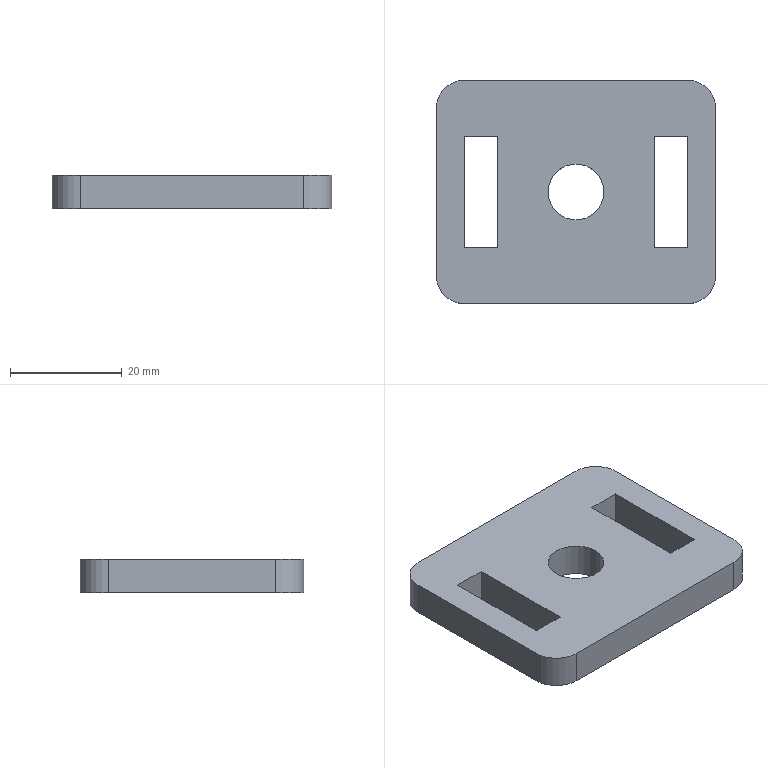Part | SolidWorks | features FlatPattern 1, SMBaseFlange 1, SheetMetal 1 | 1 solid | 20 faces | box 50 x 40 x 6 mm | volume 9960 mm3 | plane 14 | cylinder 6 | commonest cylinder face diameters 10 x6
STEP:
#1=CARTESIAN_POINT('',(-172.,0.,6.));
#2=VERTEX_POINT('',#1);
#3=CARTESIAN_POINT('',(-162.,0.,6.));
#4=VERTEX_POINT('',#3);
#5=CARTESIAN_POINT('',(-167.,0.,6.));
#6=DIRECTION('',(0.,0.,1.));
#7=DIRECTION('',(1.,0.,0.));
#8=AXIS2_PLACEMENT_3D('',#5,#6,#7);
#9=CIRCLE('',#8,5.);
#10=EDGE_CURVE('',#2,#4,#9,.T.);
#11=ORIENTED_EDGE('',*,*,#10,.T.);
#12=CARTESIAN_POINT('',(-162.,0.,0.));
#13=VERTEX_POINT('',#12);
#14=CARTESIAN_POINT('',(-162.,0.,6.));
#15=DIRECTION('',(0.,0.,-1.));
#16=VECTOR('',#15,1000.);
#17=LINE('',#14,#16);
#18=EDGE_CURVE('',#4,#13,#17,.T.);
#19=ORIENTED_EDGE('',*,*,#18,.T.);
#20=CARTESIAN_POINT('',(-172.,0.,0.));
#21=VERTEX_POINT('',#20);
#22=CARTESIAN_POINT('',(-167.,0.,0.));
#23=DIRECTION('',(0.,0.,1.));
#24=DIRECTION('',(1.,0.,0.));
#25=AXIS2_PLACEMENT_3D('',#22,#23,#24);
#26=CIRCLE('',#25,5.);
#27=EDGE_CURVE('',#21,#13,#26,.T.);
#28=ORIENTED_EDGE('',*,*,#27,.F.);
#29=CARTESIAN_POINT('',(-172.,0.,6.));
#30=DIRECTION('',(0.,0.,-1.));
#31=VECTOR('',#30,1000.);
#32=LINE('',#29,#31);
#33=EDGE_CURVE('',#2,#21,#32,.T.);
#34=ORIENTED_EDGE('',*,*,#33,.F.);
#35=EDGE_LOOP('',(#11,#19,#28,#34));
#36=FACE_OUTER_BOUND('',#35,.T.);
#37=CARTESIAN_POINT('',(-167.,0.,6.));
#38=DIRECTION('',(0.,0.,-1.));
#39=DIRECTION('',(-1.,0.,0.));
#40=AXIS2_PLACEMENT_3D('',#37,#38,#39);
#41=CYLINDRICAL_SURFACE('',#40,5.);
#42=ADVANCED_FACE('',(#36),#41,.F.);
#43=CARTESIAN_POINT('',(-147.,-20.,6.));
#44=VERTEX_POINT('',#43);
#45=CARTESIAN_POINT('',(-142.,-15.,6.));
#46=VERTEX_POINT('',#45);
#47=CARTESIAN_POINT('',(-147.,-15.,6.));
#48=DIRECTION('',(0.,0.,1.));
#49=DIRECTION('',(1.,0.,0.));
#50=AXIS2_PLACEMENT_3D('',#47,#48,#49);
#51=CIRCLE('',#50,5.);
#52=EDGE_CURVE('',#44,#46,#51,.T.);
#53=ORIENTED_EDGE('',*,*,#52,.T.);
#54=CARTESIAN_POINT('',(-142.,15.,6.));
#55=VERTEX_POINT('',#54);
#56=CARTESIAN_POINT('',(-142.,15.,6.));
#57=DIRECTION('',(0.,1.,0.));
#58=VECTOR('',#57,1000.);
#59=LINE('',#56,#58);
#60=EDGE_CURVE('',#46,#55,#59,.T.);
#61=ORIENTED_EDGE('',*,*,#60,.T.);
#62=CARTESIAN_POINT('',(-147.,20.,6.));
#63=VERTEX_POINT('',#62);
#64=CARTESIAN_POINT('',(-147.,15.,6.));
#65=DIRECTION('',(0.,0.,1.));
#66=DIRECTION('',(-1.,0.,0.));
#67=AXIS2_PLACEMENT_3D('',#64,#65,#66);
#68=CIRCLE('',#67,5.);
#69=EDGE_CURVE('',#55,#63,#68,.T.);
#70=ORIENTED_EDGE('',*,*,#69,.T.);
#71=CARTESIAN_POINT('',(-187.,20.,6.));
#72=VERTEX_POINT('',#71);
#73=CARTESIAN_POINT('',(-187.,20.,6.));
#74=DIRECTION('',(-1.,0.,0.));
#75=VECTOR('',#74,1000.);
#76=LINE('',#73,#75);
#77=EDGE_CURVE('',#63,#72,#76,.T.);
#78=ORIENTED_EDGE('',*,*,#77,.T.);
#79=CARTESIAN_POINT('',(-192.,15.,6.));
#80=VERTEX_POINT('',#79);
#81=CARTESIAN_POINT('',(-187.,15.,6.));
#82=DIRECTION('',(0.,0.,1.));
#83=DIRECTION('',(1.,0.,0.));
#84=AXIS2_PLACEMENT_3D('',#81,#82,#83);
#85=CIRCLE('',#84,5.);
#86=EDGE_CURVE('',#72,#80,#85,.T.);
#87=ORIENTED_EDGE('',*,*,#86,.T.);
#88=CARTESIAN_POINT('',(-192.,-15.,6.));
#89=VERTEX_POINT('',#88);
#90=CARTESIAN_POINT('',(-192.,15.,6.));
#91=DIRECTION('',(0.,-1.,0.));
#92=VECTOR('',#91,1000.);
#93=LINE('',#90,#92);
#94=EDGE_CURVE('',#80,#89,#93,.T.);
#95=ORIENTED_EDGE('',*,*,#94,.T.);
#96=CARTESIAN_POINT('',(-187.,-20.,6.));
#97=VERTEX_POINT('',#96);
#98=CARTESIAN_POINT('',(-187.,-15.,6.));
#99=DIRECTION('',(0.,0.,1.));
#100=DIRECTION('',(1.,0.,0.));
#101=AXIS2_PLACEMENT_3D('',#98,#99,#100);
#102=CIRCLE('',#101,5.);
#103=EDGE_CURVE('',#89,#97,#102,.T.);
#104=ORIENTED_EDGE('',*,*,#103,.T.);
#105=CARTESIAN_POINT('',(-187.,-20.,6.));
#106=DIRECTION('',(1.,0.,0.));
#107=VECTOR('',#106,1000.);
#108=LINE('',#105,#107);
#109=EDGE_CURVE('',#97,#44,#108,.T.);
#110=ORIENTED_EDGE('',*,*,#109,.T.);
#111=EDGE_LOOP('',(#53,#61,#70,#78,#87,#95,#104,#110));
#112=FACE_OUTER_BOUND('',#111,.T.);
#113=ORIENTED_EDGE('',*,*,#10,.F.);
#114=CARTESIAN_POINT('',(-167.,0.,6.));
#115=DIRECTION('',(0.,0.,1.));
#116=DIRECTION('',(1.,0.,0.));
#117=AXIS2_PLACEMENT_3D('',#114,#115,#116);
#118=CIRCLE('',#117,5.);
#119=EDGE_CURVE('',#4,#2,#118,.T.);
#120=ORIENTED_EDGE('',*,*,#119,.F.);
#121=EDGE_LOOP('',(#113,#120));
#122=FACE_BOUND('',#121,.T.);
#123=CARTESIAN_POINT('',(-181.,10.,6.));
#124=VERTEX_POINT('',#123);
#125=CARTESIAN_POINT('',(-187.,10.,6.));
#126=VERTEX_POINT('',#125);
#127=CARTESIAN_POINT('',(-181.,10.,6.));
#128=DIRECTION('',(-1.,0.,0.));
#129=VECTOR('',#128,1000.);
#130=LINE('',#127,#129);
#131=EDGE_CURVE('',#124,#126,#130,.T.);
#132=ORIENTED_EDGE('',*,*,#131,.F.);
#133=CARTESIAN_POINT('',(-181.,-10.,6.));
#134=VERTEX_POINT('',#133);
#135=CARTESIAN_POINT('',(-181.,10.,6.));
#136=DIRECTION('',(0.,1.,0.));
#137=VECTOR('',#136,1000.);
#138=LINE('',#135,#137);
#139=EDGE_CURVE('',#134,#124,#138,.T.);
#140=ORIENTED_EDGE('',*,*,#139,.F.);
#141=CARTESIAN_POINT('',(-187.,-10.,6.));
#142=VERTEX_POINT('',#141);
#143=CARTESIAN_POINT('',(-181.,-10.,6.));
#144=DIRECTION('',(1.,0.,0.));
#145=VECTOR('',#144,1000.);
#146=LINE('',#143,#145);
#147=EDGE_CURVE('',#142,#134,#146,.T.);
#148=ORIENTED_EDGE('',*,*,#147,.F.);
#149=CARTESIAN_POINT('',(-187.,10.,6.));
#150=DIRECTION('',(0.,-1.,0.));
#151=VECTOR('',#150,1000.);
#152=LINE('',#149,#151);
#153=EDGE_CURVE('',#126,#142,#152,.T.);
#154=ORIENTED_EDGE('',*,*,#153,.F.);
#155=EDGE_LOOP('',(#132,#140,#148,#154));
#156=FACE_BOUND('',#155,.T.);
#157=CARTESIAN_POINT('',(-153.,-10.,6.));
#158=VERTEX_POINT('',#157);
#159=CARTESIAN_POINT('',(-147.,-10.,6.));
#160=VERTEX_POINT('',#159);
#161=CARTESIAN_POINT('',(-153.,-10.,6.));
#162=DIRECTION('',(1.,0.,0.));
#163=VECTOR('',#162,1000.);
#164=LINE('',#161,#163);
#165=EDGE_CURVE('',#158,#160,#164,.T.);
#166=ORIENTED_EDGE('',*,*,#165,.F.);
#167=CARTESIAN_POINT('',(-153.,10.,6.));
#168=VERTEX_POINT('',#167);
#169=CARTESIAN_POINT('',(-153.,10.,6.));
#170=DIRECTION('',(0.,-1.,0.));
#171=VECTOR('',#170,1000.);
#172=LINE('',#169,#171);
#173=EDGE_CURVE('',#168,#158,#172,.T.);
#174=ORIENTED_EDGE('',*,*,#173,.F.);
#175=CARTESIAN_POINT('',(-147.,10.,6.));
#176=VERTEX_POINT('',#175);
#177=CARTESIAN_POINT('',(-153.,10.,6.));
#178=DIRECTION('',(-1.,0.,0.));
#179=VECTOR('',#178,1000.);
#180=LINE('',#177,#179);
#181=EDGE_CURVE('',#176,#168,#180,.T.);
#182=ORIENTED_EDGE('',*,*,#181,.F.);
#183=CARTESIAN_POINT('',(-147.,10.,6.));
#184=DIRECTION('',(0.,1.,0.));
#185=VECTOR('',#184,1000.);
#186=LINE('',#183,#185);
#187=EDGE_CURVE('',#160,#176,#186,.T.);
#188=ORIENTED_EDGE('',*,*,#187,.F.);
#189=EDGE_LOOP('',(#166,#174,#182,#188));
#190=FACE_BOUND('',#189,.T.);
#191=CARTESIAN_POINT('',(-147.,-15.,6.));
#192=DIRECTION('',(0.,0.,1.));
#193=DIRECTION('',(1.,0.,0.));
#194=AXIS2_PLACEMENT_3D('',#191,#192,#193);
#195=PLANE('',#194);
#196=ADVANCED_FACE('',(#112,#122,#156,#190),#195,.T.);
#197=CARTESIAN_POINT('',(-181.,-10.,0.));
#198=VERTEX_POINT('',#197);
#199=CARTESIAN_POINT('',(-181.,10.,0.));
#200=VERTEX_POINT('',#199);
#201=CARTESIAN_POINT('',(-181.,10.,0.));
#202=DIRECTION('',(0.,1.,0.));
#203=VECTOR('',#202,1000.);
#204=LINE('',#201,#203);
#205=EDGE_CURVE('',#198,#200,#204,.T.);
#206=ORIENTED_EDGE('',*,*,#205,.T.);
#207=CARTESIAN_POINT('',(-187.,10.,0.));
#208=VERTEX_POINT('',#207);
#209=CARTESIAN_POINT('',(-181.,10.,0.));
#210=DIRECTION('',(-1.,0.,0.));
#211=VECTOR('',#210,1000.);
#212=LINE('',#209,#211);
#213=EDGE_CURVE('',#200,#208,#212,.T.);
#214=ORIENTED_EDGE('',*,*,#213,.T.);
#215=CARTESIAN_POINT('',(-187.,-10.,0.));
#216=VERTEX_POINT('',#215);
#217=CARTESIAN_POINT('',(-187.,10.,0.));
#218=DIRECTION('',(0.,-1.,0.));
#219=VECTOR('',#218,1000.);
#220=LINE('',#217,#219);
#221=EDGE_CURVE('',#208,#216,#220,.T.);
#222=ORIENTED_EDGE('',*,*,#221,.T.);
#223=CARTESIAN_POINT('',(-181.,-10.,0.));
#224=DIRECTION('',(1.,0.,0.));
#225=VECTOR('',#224,1000.);
#226=LINE('',#223,#225);
#227=EDGE_CURVE('',#216,#198,#226,.T.);
#228=ORIENTED_EDGE('',*,*,#227,.T.);
#229=EDGE_LOOP('',(#206,#214,#222,#228));
#230=FACE_BOUND('',#229,.T.);
#231=CARTESIAN_POINT('',(-147.,-20.,0.));
#232=VERTEX_POINT('',#231);
#233=CARTESIAN_POINT('',(-142.,-15.,0.));
#234=VERTEX_POINT('',#233);
#235=CARTESIAN_POINT('',(-147.,-15.,0.));
#236=DIRECTION('',(0.,0.,1.));
#237=DIRECTION('',(1.,0.,0.));
#238=AXIS2_PLACEMENT_3D('',#235,#236,#237);
#239=CIRCLE('',#238,5.);
#240=EDGE_CURVE('',#232,#234,#239,.T.);
#241=ORIENTED_EDGE('',*,*,#240,.F.);
#242=CARTESIAN_POINT('',(-187.,-20.,0.));
#243=VERTEX_POINT('',#242);
#244=CARTESIAN_POINT('',(-187.,-20.,0.));
#245=DIRECTION('',(1.,0.,0.));
#246=VECTOR('',#245,1000.);
#247=LINE('',#244,#246);
#248=EDGE_CURVE('',#243,#232,#247,.T.);
#249=ORIENTED_EDGE('',*,*,#248,.F.);
#250=CARTESIAN_POINT('',(-192.,-15.,0.));
#251=VERTEX_POINT('',#250);
#252=CARTESIAN_POINT('',(-187.,-15.,0.));
#253=DIRECTION('',(0.,0.,1.));
#254=DIRECTION('',(1.,0.,0.));
#255=AXIS2_PLACEMENT_3D('',#252,#253,#254);
#256=CIRCLE('',#255,5.);
#257=EDGE_CURVE('',#251,#243,#256,.T.);
#258=ORIENTED_EDGE('',*,*,#257,.F.);
#259=CARTESIAN_POINT('',(-192.,15.,0.));
#260=VERTEX_POINT('',#259);
#261=CARTESIAN_POINT('',(-192.,15.,0.));
#262=DIRECTION('',(0.,-1.,0.));
#263=VECTOR('',#262,1000.);
#264=LINE('',#261,#263);
#265=EDGE_CURVE('',#260,#251,#264,.T.);
#266=ORIENTED_EDGE('',*,*,#265,.F.);
#267=CARTESIAN_POINT('',(-187.,20.,0.));
#268=VERTEX_POINT('',#267);
#269=CARTESIAN_POINT('',(-187.,15.,0.));
#270=DIRECTION('',(0.,0.,1.));
#271=DIRECTION('',(1.,0.,0.));
#272=AXIS2_PLACEMENT_3D('',#269,#270,#271);
#273=CIRCLE('',#272,5.);
#274=EDGE_CURVE('',#268,#260,#273,.T.);
#275=ORIENTED_EDGE('',*,*,#274,.F.);
#276=CARTESIAN_POINT('',(-147.,20.,0.));
#277=VERTEX_POINT('',#276);
#278=CARTESIAN_POINT('',(-187.,20.,0.));
#279=DIRECTION('',(-1.,0.,0.));
#280=VECTOR('',#279,1000.);
#281=LINE('',#278,#280);
#282=EDGE_CURVE('',#277,#268,#281,.T.);
#283=ORIENTED_EDGE('',*,*,#282,.F.);
#284=CARTESIAN_POINT('',(-142.,15.,0.));
#285=VERTEX_POINT('',#284);
#286=CARTESIAN_POINT('',(-147.,15.,0.));
#287=DIRECTION('',(0.,0.,1.));
#288=DIRECTION('',(-1.,0.,0.));
#289=AXIS2_PLACEMENT_3D('',#286,#287,#288);
#290=CIRCLE('',#289,5.);
#291=EDGE_CURVE('',#285,#277,#290,.T.);
#292=ORIENTED_EDGE('',*,*,#291,.F.);
#293=CARTESIAN_POINT('',(-142.,15.,0.));
#294=DIRECTION('',(0.,1.,0.));
#295=VECTOR('',#294,1000.);
#296=LINE('',#293,#295);
#297=EDGE_CURVE('',#234,#285,#296,.T.);
#298=ORIENTED_EDGE('',*,*,#297,.F.);
#299=EDGE_LOOP('',(#241,#249,#258,#266,#275,#283,#292,#298));
#300=FACE_OUTER_BOUND('',#299,.T.);
#301=ORIENTED_EDGE('',*,*,#27,.T.);
#302=CARTESIAN_POINT('',(-167.,0.,0.));
#303=DIRECTION('',(0.,0.,1.));
#304=DIRECTION('',(1.,0.,0.));
#305=AXIS2_PLACEMENT_3D('',#302,#303,#304);
#306=CIRCLE('',#305,5.);
#307=EDGE_CURVE('',#13,#21,#306,.T.);
#308=ORIENTED_EDGE('',*,*,#307,.T.);
#309=EDGE_LOOP('',(#301,#308));
#310=FACE_BOUND('',#309,.T.);
#311=CARTESIAN_POINT('',(-153.,10.,0.));
#312=VERTEX_POINT('',#311);
#313=CARTESIAN_POINT('',(-153.,-10.,0.));
#314=VERTEX_POINT('',#313);
#315=CARTESIAN_POINT('',(-153.,10.,0.));
#316=DIRECTION('',(0.,-1.,0.));
#317=VECTOR('',#316,1000.);
#318=LINE('',#315,#317);
#319=EDGE_CURVE('',#312,#314,#318,.T.);
#320=ORIENTED_EDGE('',*,*,#319,.T.);
#321=CARTESIAN_POINT('',(-147.,-10.,0.));
#322=VERTEX_POINT('',#321);
#323=CARTESIAN_POINT('',(-153.,-10.,0.));
#324=DIRECTION('',(1.,0.,0.));
#325=VECTOR('',#324,1000.);
#326=LINE('',#323,#325);
#327=EDGE_CURVE('',#314,#322,#326,.T.);
#328=ORIENTED_EDGE('',*,*,#327,.T.);
#329=CARTESIAN_POINT('',(-147.,10.,0.));
#330=VERTEX_POINT('',#329);
#331=CARTESIAN_POINT('',(-147.,10.,0.));
#332=DIRECTION('',(0.,1.,0.));
#333=VECTOR('',#332,1000.);
#334=LINE('',#331,#333);
#335=EDGE_CURVE('',#322,#330,#334,.T.);
#336=ORIENTED_EDGE('',*,*,#335,.T.);
#337=CARTESIAN_POINT('',(-153.,10.,0.));
#338=DIRECTION('',(-1.,0.,0.));
#339=VECTOR('',#338,1000.);
#340=LINE('',#337,#339);
#341=EDGE_CURVE('',#330,#312,#340,.T.);
#342=ORIENTED_EDGE('',*,*,#341,.T.);
#343=EDGE_LOOP('',(#320,#328,#336,#342));
#344=FACE_BOUND('',#343,.T.);
#345=CARTESIAN_POINT('',(-147.,-15.,0.));
#346=DIRECTION('',(0.,0.,1.));
#347=DIRECTION('',(1.,0.,0.));
#348=AXIS2_PLACEMENT_3D('',#345,#346,#347);
#349=PLANE('',#348);
#350=ADVANCED_FACE('',(#230,#300,#310,#344),#349,.F.);
#351=ORIENTED_EDGE('',*,*,#240,.T.);
#352=CARTESIAN_POINT('',(-142.,-15.,6.));
#353=DIRECTION('',(0.,0.,-1.));
#354=VECTOR('',#353,1000.);
#355=LINE('',#352,#354);
#356=EDGE_CURVE('',#46,#234,#355,.T.);
#357=ORIENTED_EDGE('',*,*,#356,.F.);
#358=ORIENTED_EDGE('',*,*,#52,.F.);
#359=CARTESIAN_POINT('',(-147.,-20.,6.));
#360=DIRECTION('',(0.,0.,-1.));
#361=VECTOR('',#360,1000.);
#362=LINE('',#359,#361);
#363=EDGE_CURVE('',#44,#232,#362,.T.);
#364=ORIENTED_EDGE('',*,*,#363,.T.);
#365=EDGE_LOOP('',(#351,#357,#358,#364));
#366=FACE_OUTER_BOUND('',#365,.T.);
#367=CARTESIAN_POINT('',(-147.,-15.,6.));
#368=DIRECTION('',(0.,0.,-1.));
#369=DIRECTION('',(-1.,0.,0.));
#370=AXIS2_PLACEMENT_3D('',#367,#368,#369);
#371=CYLINDRICAL_SURFACE('',#370,5.);
#372=ADVANCED_FACE('',(#366),#371,.T.);
#373=ORIENTED_EDGE('',*,*,#297,.T.);
#374=CARTESIAN_POINT('',(-142.,15.,6.));
#375=DIRECTION('',(0.,0.,-1.));
#376=VECTOR('',#375,1000.);
#377=LINE('',#374,#376);
#378=EDGE_CURVE('',#55,#285,#377,.T.);
#379=ORIENTED_EDGE('',*,*,#378,.F.);
#380=ORIENTED_EDGE('',*,*,#60,.F.);
#381=ORIENTED_EDGE('',*,*,#356,.T.);
#382=EDGE_LOOP('',(#373,#379,#380,#381));
#383=FACE_OUTER_BOUND('',#382,.T.);
#384=CARTESIAN_POINT('',(-142.,15.,6.));
#385=DIRECTION('',(-1.,0.,0.));
#386=DIRECTION('',(0.,0.,1.));
#387=AXIS2_PLACEMENT_3D('',#384,#385,#386);
#388=PLANE('',#387);
#389=ADVANCED_FACE('',(#383),#388,.F.);
#390=ORIENTED_EDGE('',*,*,#291,.T.);
#391=CARTESIAN_POINT('',(-147.,20.,6.));
#392=DIRECTION('',(0.,0.,-1.));
#393=VECTOR('',#392,1000.);
#394=LINE('',#391,#393);
#395=EDGE_CURVE('',#63,#277,#394,.T.);
#396=ORIENTED_EDGE('',*,*,#395,.F.);
#397=ORIENTED_EDGE('',*,*,#69,.F.);
#398=ORIENTED_EDGE('',*,*,#378,.T.);
#399=EDGE_LOOP('',(#390,#396,#397,#398));
#400=FACE_OUTER_BOUND('',#399,.T.);
#401=CARTESIAN_POINT('',(-147.,15.,6.));
#402=DIRECTION('',(0.,0.,-1.));
#403=DIRECTION('',(-1.,0.,0.));
#404=AXIS2_PLACEMENT_3D('',#401,#402,#403);
#405=CYLINDRICAL_SURFACE('',#404,5.);
#406=ADVANCED_FACE('',(#400),#405,.T.);
#407=ORIENTED_EDGE('',*,*,#282,.T.);
#408=CARTESIAN_POINT('',(-187.,20.,6.));
#409=DIRECTION('',(0.,0.,-1.));
#410=VECTOR('',#409,1000.);
#411=LINE('',#408,#410);
#412=EDGE_CURVE('',#72,#268,#411,.T.);
#413=ORIENTED_EDGE('',*,*,#412,.F.);
#414=ORIENTED_EDGE('',*,*,#77,.F.);
#415=ORIENTED_EDGE('',*,*,#395,.T.);
#416=EDGE_LOOP('',(#407,#413,#414,#415));
#417=FACE_OUTER_BOUND('',#416,.T.);
#418=CARTESIAN_POINT('',(-187.,20.,6.));
#419=DIRECTION('',(0.,-1.,0.));
#420=DIRECTION('',(0.,0.,-1.));
#421=AXIS2_PLACEMENT_3D('',#418,#419,#420);
#422=PLANE('',#421);
#423=ADVANCED_FACE('',(#417),#422,.F.);
#424=ORIENTED_EDGE('',*,*,#274,.T.);
#425=CARTESIAN_POINT('',(-192.,15.,6.));
#426=DIRECTION('',(0.,0.,-1.));
#427=VECTOR('',#426,1000.);
#428=LINE('',#425,#427);
#429=EDGE_CURVE('',#80,#260,#428,.T.);
#430=ORIENTED_EDGE('',*,*,#429,.F.);
#431=ORIENTED_EDGE('',*,*,#86,.F.);
#432=ORIENTED_EDGE('',*,*,#412,.T.);
#433=EDGE_LOOP('',(#424,#430,#431,#432));
#434=FACE_OUTER_BOUND('',#433,.T.);
#435=CARTESIAN_POINT('',(-187.,15.,6.));
#436=DIRECTION('',(0.,0.,-1.));
#437=DIRECTION('',(-1.,0.,0.));
#438=AXIS2_PLACEMENT_3D('',#435,#436,#437);
#439=CYLINDRICAL_SURFACE('',#438,5.);
#440=ADVANCED_FACE('',(#434),#439,.T.);
#441=ORIENTED_EDGE('',*,*,#265,.T.);
#442=CARTESIAN_POINT('',(-192.,-15.,6.));
#443=DIRECTION('',(0.,0.,-1.));
#444=VECTOR('',#443,1000.);
#445=LINE('',#442,#444);
#446=EDGE_CURVE('',#89,#251,#445,.T.);
#447=ORIENTED_EDGE('',*,*,#446,.F.);
#448=ORIENTED_EDGE('',*,*,#94,.F.);
#449=ORIENTED_EDGE('',*,*,#429,.T.);
#450=EDGE_LOOP('',(#441,#447,#448,#449));
#451=FACE_OUTER_BOUND('',#450,.T.);
#452=CARTESIAN_POINT('',(-192.,15.,6.));
#453=DIRECTION('',(1.,0.,0.));
#454=DIRECTION('',(0.,0.,-1.));
#455=AXIS2_PLACEMENT_3D('',#452,#453,#454);
#456=PLANE('',#455);
#457=ADVANCED_FACE('',(#451),#456,.F.);
#458=ORIENTED_EDGE('',*,*,#257,.T.);
#459=CARTESIAN_POINT('',(-187.,-20.,6.));
#460=DIRECTION('',(0.,0.,-1.));
#461=VECTOR('',#460,1000.);
#462=LINE('',#459,#461);
#463=EDGE_CURVE('',#97,#243,#462,.T.);
#464=ORIENTED_EDGE('',*,*,#463,.F.);
#465=ORIENTED_EDGE('',*,*,#103,.F.);
#466=ORIENTED_EDGE('',*,*,#446,.T.);
#467=EDGE_LOOP('',(#458,#464,#465,#466));
#468=FACE_OUTER_BOUND('',#467,.T.);
#469=CARTESIAN_POINT('',(-187.,-15.,6.));
#470=DIRECTION('',(0.,0.,-1.));
#471=DIRECTION('',(-1.,0.,0.));
#472=AXIS2_PLACEMENT_3D('',#469,#470,#471);
#473=CYLINDRICAL_SURFACE('',#472,5.);
#474=ADVANCED_FACE('',(#468),#473,.T.);
#475=ORIENTED_EDGE('',*,*,#248,.T.);
#476=ORIENTED_EDGE('',*,*,#363,.F.);
#477=ORIENTED_EDGE('',*,*,#109,.F.);
#478=ORIENTED_EDGE('',*,*,#463,.T.);
#479=EDGE_LOOP('',(#475,#476,#477,#478));
#480=FACE_OUTER_BOUND('',#479,.T.);
#481=CARTESIAN_POINT('',(-187.,-20.,6.));
#482=DIRECTION('',(0.,1.,0.));
#483=DIRECTION('',(0.,0.,1.));
#484=AXIS2_PLACEMENT_3D('',#481,#482,#483);
#485=PLANE('',#484);
#486=ADVANCED_FACE('',(#480),#485,.F.);
#487=ORIENTED_EDGE('',*,*,#18,.F.);
#488=ORIENTED_EDGE('',*,*,#119,.T.);
#489=ORIENTED_EDGE('',*,*,#33,.T.);
#490=ORIENTED_EDGE('',*,*,#307,.F.);
#491=EDGE_LOOP('',(#487,#488,#489,#490));
#492=FACE_OUTER_BOUND('',#491,.T.);
#493=CARTESIAN_POINT('',(-167.,0.,6.));
#494=DIRECTION('',(0.,0.,-1.));
#495=DIRECTION('',(-1.,0.,0.));
#496=AXIS2_PLACEMENT_3D('',#493,#494,#495);
#497=CYLINDRICAL_SURFACE('',#496,5.);
#498=ADVANCED_FACE('',(#492),#497,.F.);
#499=ORIENTED_EDGE('',*,*,#205,.F.);
#500=CARTESIAN_POINT('',(-181.,-10.,6.));
#501=DIRECTION('',(0.,0.,-1.));
#502=VECTOR('',#501,1000.);
#503=LINE('',#500,#502);
#504=EDGE_CURVE('',#134,#198,#503,.T.);
#505=ORIENTED_EDGE('',*,*,#504,.F.);
#506=ORIENTED_EDGE('',*,*,#139,.T.);
#507=CARTESIAN_POINT('',(-181.,10.,6.));
#508=DIRECTION('',(0.,0.,-1.));
#509=VECTOR('',#508,1000.);
#510=LINE('',#507,#509);
#511=EDGE_CURVE('',#124,#200,#510,.T.);
#512=ORIENTED_EDGE('',*,*,#511,.T.);
#513=EDGE_LOOP('',(#499,#505,#506,#512));
#514=FACE_OUTER_BOUND('',#513,.T.);
#515=CARTESIAN_POINT('',(-181.,10.,6.));
#516=DIRECTION('',(-1.,0.,0.));
#517=DIRECTION('',(0.,0.,1.));
#518=AXIS2_PLACEMENT_3D('',#515,#516,#517);
#519=PLANE('',#518);
#520=ADVANCED_FACE('',(#514),#519,.T.);
#521=ORIENTED_EDGE('',*,*,#213,.F.);
#522=ORIENTED_EDGE('',*,*,#511,.F.);
#523=ORIENTED_EDGE('',*,*,#131,.T.);
#524=CARTESIAN_POINT('',(-187.,10.,6.));
#525=DIRECTION('',(0.,0.,-1.));
#526=VECTOR('',#525,1000.);
#527=LINE('',#524,#526);
#528=EDGE_CURVE('',#126,#208,#527,.T.);
#529=ORIENTED_EDGE('',*,*,#528,.T.);
#530=EDGE_LOOP('',(#521,#522,#523,#529));
#531=FACE_OUTER_BOUND('',#530,.T.);
#532=CARTESIAN_POINT('',(-181.,10.,6.));
#533=DIRECTION('',(0.,-1.,0.));
#534=DIRECTION('',(0.,0.,-1.));
#535=AXIS2_PLACEMENT_3D('',#532,#533,#534);
#536=PLANE('',#535);
#537=ADVANCED_FACE('',(#531),#536,.T.);
#538=ORIENTED_EDGE('',*,*,#221,.F.);
#539=ORIENTED_EDGE('',*,*,#528,.F.);
#540=ORIENTED_EDGE('',*,*,#153,.T.);
#541=CARTESIAN_POINT('',(-187.,-10.,6.));
#542=DIRECTION('',(0.,0.,-1.));
#543=VECTOR('',#542,1000.);
#544=LINE('',#541,#543);
#545=EDGE_CURVE('',#142,#216,#544,.T.);
#546=ORIENTED_EDGE('',*,*,#545,.T.);
#547=EDGE_LOOP('',(#538,#539,#540,#546));
#548=FACE_OUTER_BOUND('',#547,.T.);
#549=CARTESIAN_POINT('',(-187.,10.,6.));
#550=DIRECTION('',(1.,0.,0.));
#551=DIRECTION('',(0.,0.,-1.));
#552=AXIS2_PLACEMENT_3D('',#549,#550,#551);
#553=PLANE('',#552);
#554=ADVANCED_FACE('',(#548),#553,.T.);
#555=ORIENTED_EDGE('',*,*,#227,.F.);
#556=ORIENTED_EDGE('',*,*,#545,.F.);
#557=ORIENTED_EDGE('',*,*,#147,.T.);
#558=ORIENTED_EDGE('',*,*,#504,.T.);
#559=EDGE_LOOP('',(#555,#556,#557,#558));
#560=FACE_OUTER_BOUND('',#559,.T.);
#561=CARTESIAN_POINT('',(-181.,-10.,6.));
#562=DIRECTION('',(0.,1.,0.));
#563=DIRECTION('',(0.,0.,1.));
#564=AXIS2_PLACEMENT_3D('',#561,#562,#563);
#565=PLANE('',#564);
#566=ADVANCED_FACE('',(#560),#565,.T.);
#567=ORIENTED_EDGE('',*,*,#319,.F.);
#568=CARTESIAN_POINT('',(-153.,10.,6.));
#569=DIRECTION('',(0.,0.,-1.));
#570=VECTOR('',#569,1000.);
#571=LINE('',#568,#570);
#572=EDGE_CURVE('',#168,#312,#571,.T.);
#573=ORIENTED_EDGE('',*,*,#572,.F.);
#574=ORIENTED_EDGE('',*,*,#173,.T.);
#575=CARTESIAN_POINT('',(-153.,-10.,6.));
#576=DIRECTION('',(0.,0.,-1.));
#577=VECTOR('',#576,1000.);
#578=LINE('',#575,#577);
#579=EDGE_CURVE('',#158,#314,#578,.T.);
#580=ORIENTED_EDGE('',*,*,#579,.T.);
#581=EDGE_LOOP('',(#567,#573,#574,#580));
#582=FACE_OUTER_BOUND('',#581,.T.);
#583=CARTESIAN_POINT('',(-153.,10.,6.));
#584=DIRECTION('',(1.,0.,0.));
#585=DIRECTION('',(0.,0.,-1.));
#586=AXIS2_PLACEMENT_3D('',#583,#584,#585);
#587=PLANE('',#586);
#588=ADVANCED_FACE('',(#582),#587,.T.);
#589=ORIENTED_EDGE('',*,*,#327,.F.);
#590=ORIENTED_EDGE('',*,*,#579,.F.);
#591=ORIENTED_EDGE('',*,*,#165,.T.);
#592=CARTESIAN_POINT('',(-147.,-10.,6.));
#593=DIRECTION('',(0.,0.,-1.));
#594=VECTOR('',#593,1000.);
#595=LINE('',#592,#594);
#596=EDGE_CURVE('',#160,#322,#595,.T.);
#597=ORIENTED_EDGE('',*,*,#596,.T.);
#598=EDGE_LOOP('',(#589,#590,#591,#597));
#599=FACE_OUTER_BOUND('',#598,.T.);
#600=CARTESIAN_POINT('',(-153.,-10.,6.));
#601=DIRECTION('',(0.,1.,0.));
#602=DIRECTION('',(0.,0.,1.));
#603=AXIS2_PLACEMENT_3D('',#600,#601,#602);
#604=PLANE('',#603);
#605=ADVANCED_FACE('',(#599),#604,.T.);
#606=ORIENTED_EDGE('',*,*,#335,.F.);
#607=ORIENTED_EDGE('',*,*,#596,.F.);
#608=ORIENTED_EDGE('',*,*,#187,.T.);
#609=CARTESIAN_POINT('',(-147.,10.,6.));
#610=DIRECTION('',(0.,0.,-1.));
#611=VECTOR('',#610,1000.);
#612=LINE('',#609,#611);
#613=EDGE_CURVE('',#176,#330,#612,.T.);
#614=ORIENTED_EDGE('',*,*,#613,.T.);
#615=EDGE_LOOP('',(#606,#607,#608,#614));
#616=FACE_OUTER_BOUND('',#615,.T.);
#617=CARTESIAN_POINT('',(-147.,10.,6.));
#618=DIRECTION('',(-1.,0.,0.));
#619=DIRECTION('',(0.,0.,1.));
#620=AXIS2_PLACEMENT_3D('',#617,#618,#619);
#621=PLANE('',#620);
#622=ADVANCED_FACE('',(#616),#621,.T.);
#623=ORIENTED_EDGE('',*,*,#341,.F.);
#624=ORIENTED_EDGE('',*,*,#613,.F.);
#625=ORIENTED_EDGE('',*,*,#181,.T.);
#626=ORIENTED_EDGE('',*,*,#572,.T.);
#627=EDGE_LOOP('',(#623,#624,#625,#626));
#628=FACE_OUTER_BOUND('',#627,.T.);
#629=CARTESIAN_POINT('',(-153.,10.,6.));
#630=DIRECTION('',(0.,-1.,0.));
#631=DIRECTION('',(0.,0.,-1.));
#632=AXIS2_PLACEMENT_3D('',#629,#630,#631);
#633=PLANE('',#632);
#634=ADVANCED_FACE('',(#628),#633,.T.);
#635=CLOSED_SHELL('',(#42,#196,#350,#372,#389,#406,#423,#440,#457,#474,#486,#498,#520,#537,#554,#566,#588,#605,#622,#634));
#636=MANIFOLD_SOLID_BREP('',#635);
#637=CARTESIAN_POINT('',(0.,0.,0.));
#638=DIRECTION('',(0.,0.,1.));
#639=DIRECTION('',(1.,0.,0.));
#640=AXIS2_PLACEMENT_3D('',#637,#638,#639);
#641=(LENGTH_UNIT()NAMED_UNIT(*)SI_UNIT(.MILLI.,.METRE.));
#642=UNCERTAINTY_MEASURE_WITH_UNIT(LENGTH_MEASURE(0.00001),#641,'','');
#643=(NAMED_UNIT(*)PLANE_ANGLE_UNIT()SI_UNIT($,.RADIAN.));
#644=(NAMED_UNIT(*)SI_UNIT($,.STERADIAN.)SOLID_ANGLE_UNIT());
#645=(GEOMETRIC_REPRESENTATION_CONTEXT(3)GLOBAL_UNCERTAINTY_ASSIGNED_CONTEXT((#642))GLOBAL_UNIT_ASSIGNED_CONTEXT((#641,#643,#644))REPRESENTATION_CONTEXT('',''));
#646=ADVANCED_BREP_SHAPE_REPRESENTATION('',(#636,#640),#645);